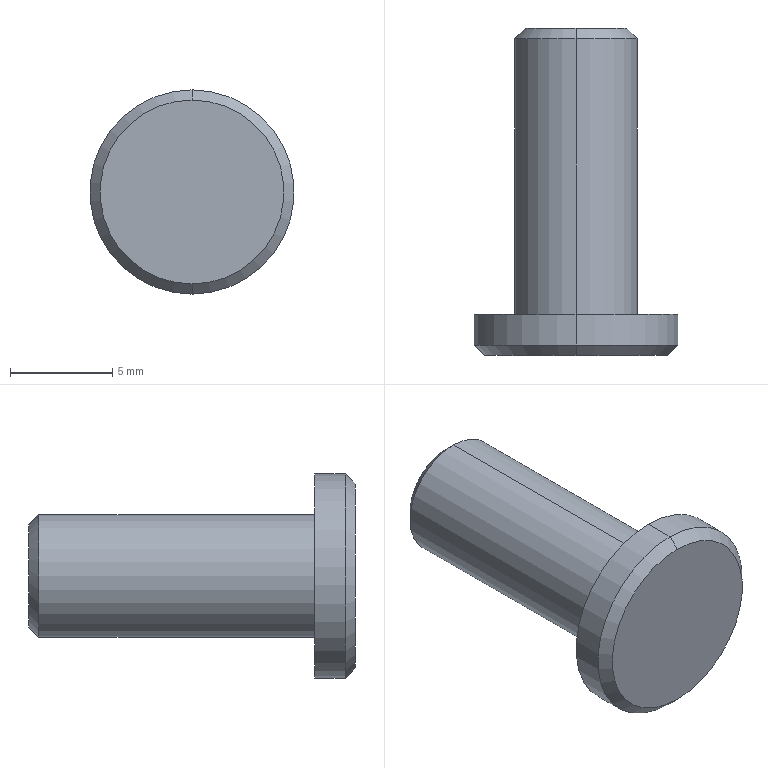Part | SolidWorks | features Chamfer 1, Extrusion 1, ICE 1 | 1 solid | 11 faces | box 10 x 16 x 10 mm | volume 546.899 mm3 | cone 4 | cylinder 4 | plane 3 | commonest cylinder face diameters 6 x2 10 x2
STEP:
#1=CARTESIAN_POINT('',(0.,0.,-4.5));
#2=VERTEX_POINT('',#1);
#3=CARTESIAN_POINT('',(0.,0.,4.5));
#4=VERTEX_POINT('',#3);
#5=CARTESIAN_POINT('',(0.,0.,0.));
#6=DIRECTION('',(0.,-1.,0.));
#7=DIRECTION('',(0.,0.,1.));
#8=AXIS2_PLACEMENT_3D('',#5,#6,#7);
#9=CIRCLE('',#8,4.5);
#10=EDGE_CURVE('',#2,#4,#9,.T.);
#11=ORIENTED_EDGE('',*,*,#10,.F.);
#12=CARTESIAN_POINT('',(0.,0.5,-5.));
#13=VERTEX_POINT('',#12);
#14=CARTESIAN_POINT('',(0.,0.5,-5.));
#15=DIRECTION('',(0.,0.7071,-0.7071));
#16=VECTOR('',#15,1000.);
#17=LINE('',#14,#16);
#18=EDGE_CURVE('',#2,#13,#17,.T.);
#19=ORIENTED_EDGE('',*,*,#18,.T.);
#20=CARTESIAN_POINT('',(0.,0.5,5.));
#21=VERTEX_POINT('',#20);
#22=CARTESIAN_POINT('',(0.,0.5,0.));
#23=DIRECTION('',(0.,1.,0.));
#24=DIRECTION('',(0.,0.,1.));
#25=AXIS2_PLACEMENT_3D('',#22,#23,#24);
#26=CIRCLE('',#25,5.);
#27=EDGE_CURVE('',#21,#13,#26,.T.);
#28=ORIENTED_EDGE('',*,*,#27,.F.);
#29=CARTESIAN_POINT('',(0.,0.5,5.));
#30=DIRECTION('',(0.,0.7071,0.7071));
#31=VECTOR('',#30,1000.);
#32=LINE('',#29,#31);
#33=EDGE_CURVE('',#4,#21,#32,.T.);
#34=ORIENTED_EDGE('',*,*,#33,.F.);
#35=EDGE_LOOP('',(#11,#19,#28,#34));
#36=FACE_OUTER_BOUND('',#35,.T.);
#37=CARTESIAN_POINT('',(0.,0.5,0.));
#38=DIRECTION('',(0.,1.,0.));
#39=DIRECTION('',(0.,0.,1.));
#40=AXIS2_PLACEMENT_3D('',#37,#38,#39);
#41=CONICAL_SURFACE('',#40,5.,0.7854);
#42=ADVANCED_FACE('',(#36),#41,.T.);
#43=CARTESIAN_POINT('',(0.,16.,2.5));
#44=VERTEX_POINT('',#43);
#45=CARTESIAN_POINT('',(0.,16.,-2.5));
#46=VERTEX_POINT('',#45);
#47=CARTESIAN_POINT('',(0.,16.,0.));
#48=DIRECTION('',(0.,1.,0.));
#49=DIRECTION('',(0.,0.,1.));
#50=AXIS2_PLACEMENT_3D('',#47,#48,#49);
#51=CIRCLE('',#50,2.5);
#52=EDGE_CURVE('',#44,#46,#51,.T.);
#53=ORIENTED_EDGE('',*,*,#52,.F.);
#54=CARTESIAN_POINT('',(0.,15.5,3.));
#55=VERTEX_POINT('',#54);
#56=CARTESIAN_POINT('',(0.,16.,2.5));
#57=DIRECTION('',(0.,-0.7071,0.7071));
#58=VECTOR('',#57,1000.);
#59=LINE('',#56,#58);
#60=EDGE_CURVE('',#44,#55,#59,.T.);
#61=ORIENTED_EDGE('',*,*,#60,.T.);
#62=CARTESIAN_POINT('',(0.,15.5,-3.));
#63=VERTEX_POINT('',#62);
#64=CARTESIAN_POINT('',(0.,15.5,0.));
#65=DIRECTION('',(0.,-1.,0.));
#66=DIRECTION('',(0.,0.,1.));
#67=AXIS2_PLACEMENT_3D('',#64,#65,#66);
#68=CIRCLE('',#67,3.);
#69=EDGE_CURVE('',#63,#55,#68,.T.);
#70=ORIENTED_EDGE('',*,*,#69,.F.);
#71=CARTESIAN_POINT('',(0.,16.,-2.5));
#72=DIRECTION('',(0.,-0.7071,-0.7071));
#73=VECTOR('',#72,1000.);
#74=LINE('',#71,#73);
#75=EDGE_CURVE('',#46,#63,#74,.T.);
#76=ORIENTED_EDGE('',*,*,#75,.F.);
#77=EDGE_LOOP('',(#53,#61,#70,#76));
#78=FACE_OUTER_BOUND('',#77,.T.);
#79=CARTESIAN_POINT('',(0.,16.,0.));
#80=DIRECTION('',(0.,-1.,0.));
#81=DIRECTION('',(0.,0.,-1.));
#82=AXIS2_PLACEMENT_3D('',#79,#80,#81);
#83=CONICAL_SURFACE('',#82,2.5,0.7854);
#84=ADVANCED_FACE('',(#78),#83,.T.);
#85=ORIENTED_EDGE('',*,*,#69,.T.);
#86=CARTESIAN_POINT('',(0.,2.,3.));
#87=VERTEX_POINT('',#86);
#88=CARTESIAN_POINT('',(0.,16.,3.));
#89=DIRECTION('',(0.,-1.,0.));
#90=VECTOR('',#89,1000.);
#91=LINE('',#88,#90);
#92=EDGE_CURVE('',#55,#87,#91,.T.);
#93=ORIENTED_EDGE('',*,*,#92,.T.);
#94=CARTESIAN_POINT('',(0.,2.,-3.));
#95=VERTEX_POINT('',#94);
#96=CARTESIAN_POINT('',(0.,2.,0.));
#97=DIRECTION('',(0.,1.,0.));
#98=DIRECTION('',(0.,0.,1.));
#99=AXIS2_PLACEMENT_3D('',#96,#97,#98);
#100=CIRCLE('',#99,3.);
#101=EDGE_CURVE('',#87,#95,#100,.T.);
#102=ORIENTED_EDGE('',*,*,#101,.T.);
#103=CARTESIAN_POINT('',(0.,16.,-3.));
#104=DIRECTION('',(0.,-1.,0.));
#105=VECTOR('',#104,1000.);
#106=LINE('',#103,#105);
#107=EDGE_CURVE('',#63,#95,#106,.T.);
#108=ORIENTED_EDGE('',*,*,#107,.F.);
#109=EDGE_LOOP('',(#85,#93,#102,#108));
#110=FACE_OUTER_BOUND('',#109,.T.);
#111=CARTESIAN_POINT('',(0.,16.,0.));
#112=DIRECTION('',(0.,-1.,0.));
#113=DIRECTION('',(0.,0.,-1.));
#114=AXIS2_PLACEMENT_3D('',#111,#112,#113);
#115=CYLINDRICAL_SURFACE('',#114,3.);
#116=ADVANCED_FACE('',(#110),#115,.T.);
#117=CARTESIAN_POINT('',(0.,2.,5.));
#118=VERTEX_POINT('',#117);
#119=CARTESIAN_POINT('',(0.,2.,-5.));
#120=VERTEX_POINT('',#119);
#121=CARTESIAN_POINT('',(0.,2.,0.));
#122=DIRECTION('',(0.,1.,0.));
#123=DIRECTION('',(0.,0.,1.));
#124=AXIS2_PLACEMENT_3D('',#121,#122,#123);
#125=CIRCLE('',#124,5.);
#126=EDGE_CURVE('',#118,#120,#125,.T.);
#127=ORIENTED_EDGE('',*,*,#126,.F.);
#128=CARTESIAN_POINT('',(0.,2.,5.));
#129=DIRECTION('',(0.,-1.,0.));
#130=VECTOR('',#129,1000.);
#131=LINE('',#128,#130);
#132=EDGE_CURVE('',#118,#21,#131,.T.);
#133=ORIENTED_EDGE('',*,*,#132,.T.);
#134=ORIENTED_EDGE('',*,*,#27,.T.);
#135=CARTESIAN_POINT('',(0.,2.,-5.));
#136=DIRECTION('',(0.,-1.,0.));
#137=VECTOR('',#136,1000.);
#138=LINE('',#135,#137);
#139=EDGE_CURVE('',#120,#13,#138,.T.);
#140=ORIENTED_EDGE('',*,*,#139,.F.);
#141=EDGE_LOOP('',(#127,#133,#134,#140));
#142=FACE_OUTER_BOUND('',#141,.T.);
#143=CARTESIAN_POINT('',(0.,2.,0.));
#144=DIRECTION('',(0.,-1.,0.));
#145=DIRECTION('',(0.,0.,-1.));
#146=AXIS2_PLACEMENT_3D('',#143,#144,#145);
#147=CYLINDRICAL_SURFACE('',#146,5.);
#148=ADVANCED_FACE('',(#142),#147,.T.);
#149=ORIENTED_EDGE('',*,*,#132,.F.);
#150=CARTESIAN_POINT('',(0.,2.,0.));
#151=DIRECTION('',(0.,1.,0.));
#152=DIRECTION('',(0.,0.,1.));
#153=AXIS2_PLACEMENT_3D('',#150,#151,#152);
#154=CIRCLE('',#153,5.);
#155=EDGE_CURVE('',#120,#118,#154,.T.);
#156=ORIENTED_EDGE('',*,*,#155,.F.);
#157=ORIENTED_EDGE('',*,*,#139,.T.);
#158=CARTESIAN_POINT('',(0.,0.5,0.));
#159=DIRECTION('',(0.,1.,0.));
#160=DIRECTION('',(0.,0.,1.));
#161=AXIS2_PLACEMENT_3D('',#158,#159,#160);
#162=CIRCLE('',#161,5.);
#163=EDGE_CURVE('',#13,#21,#162,.T.);
#164=ORIENTED_EDGE('',*,*,#163,.T.);
#165=EDGE_LOOP('',(#149,#156,#157,#164));
#166=FACE_OUTER_BOUND('',#165,.T.);
#167=CARTESIAN_POINT('',(0.,2.,0.));
#168=DIRECTION('',(0.,-1.,0.));
#169=DIRECTION('',(0.,0.,-1.));
#170=AXIS2_PLACEMENT_3D('',#167,#168,#169);
#171=CYLINDRICAL_SURFACE('',#170,5.);
#172=ADVANCED_FACE('',(#166),#171,.T.);
#173=CARTESIAN_POINT('',(0.,2.,0.));
#174=DIRECTION('',(0.,1.,0.));
#175=DIRECTION('',(0.,0.,1.));
#176=AXIS2_PLACEMENT_3D('',#173,#174,#175);
#177=CIRCLE('',#176,3.);
#178=EDGE_CURVE('',#95,#87,#177,.T.);
#179=ORIENTED_EDGE('',*,*,#178,.F.);
#180=ORIENTED_EDGE('',*,*,#101,.F.);
#181=EDGE_LOOP('',(#179,#180));
#182=FACE_BOUND('',#181,.T.);
#183=ORIENTED_EDGE('',*,*,#155,.T.);
#184=ORIENTED_EDGE('',*,*,#126,.T.);
#185=EDGE_LOOP('',(#183,#184));
#186=FACE_OUTER_BOUND('',#185,.T.);
#187=CARTESIAN_POINT('',(0.,2.,0.));
#188=DIRECTION('',(0.,1.,0.));
#189=DIRECTION('',(0.,0.,1.));
#190=AXIS2_PLACEMENT_3D('',#187,#188,#189);
#191=PLANE('',#190);
#192=ADVANCED_FACE('',(#182,#186),#191,.T.);
#193=CARTESIAN_POINT('',(0.,0.,0.));
#194=DIRECTION('',(0.,-1.,0.));
#195=DIRECTION('',(0.,0.,1.));
#196=AXIS2_PLACEMENT_3D('',#193,#194,#195);
#197=CIRCLE('',#196,4.5);
#198=EDGE_CURVE('',#4,#2,#197,.T.);
#199=ORIENTED_EDGE('',*,*,#198,.T.);
#200=ORIENTED_EDGE('',*,*,#10,.T.);
#201=EDGE_LOOP('',(#199,#200));
#202=FACE_OUTER_BOUND('',#201,.T.);
#203=CARTESIAN_POINT('',(0.,0.,0.));
#204=DIRECTION('',(0.,1.,0.));
#205=DIRECTION('',(0.,0.,1.));
#206=AXIS2_PLACEMENT_3D('',#203,#204,#205);
#207=PLANE('',#206);
#208=ADVANCED_FACE('',(#202),#207,.F.);
#209=ORIENTED_EDGE('',*,*,#92,.F.);
#210=CARTESIAN_POINT('',(0.,15.5,0.));
#211=DIRECTION('',(0.,-1.,0.));
#212=DIRECTION('',(0.,0.,1.));
#213=AXIS2_PLACEMENT_3D('',#210,#211,#212);
#214=CIRCLE('',#213,3.);
#215=EDGE_CURVE('',#55,#63,#214,.T.);
#216=ORIENTED_EDGE('',*,*,#215,.T.);
#217=ORIENTED_EDGE('',*,*,#107,.T.);
#218=ORIENTED_EDGE('',*,*,#178,.T.);
#219=EDGE_LOOP('',(#209,#216,#217,#218));
#220=FACE_OUTER_BOUND('',#219,.T.);
#221=CARTESIAN_POINT('',(0.,16.,0.));
#222=DIRECTION('',(0.,-1.,0.));
#223=DIRECTION('',(0.,0.,-1.));
#224=AXIS2_PLACEMENT_3D('',#221,#222,#223);
#225=CYLINDRICAL_SURFACE('',#224,3.);
#226=ADVANCED_FACE('',(#220),#225,.T.);
#227=CARTESIAN_POINT('',(0.,16.,0.));
#228=DIRECTION('',(0.,1.,0.));
#229=DIRECTION('',(0.,0.,1.));
#230=AXIS2_PLACEMENT_3D('',#227,#228,#229);
#231=CIRCLE('',#230,2.5);
#232=EDGE_CURVE('',#46,#44,#231,.T.);
#233=ORIENTED_EDGE('',*,*,#232,.T.);
#234=ORIENTED_EDGE('',*,*,#52,.T.);
#235=EDGE_LOOP('',(#233,#234));
#236=FACE_OUTER_BOUND('',#235,.T.);
#237=CARTESIAN_POINT('',(0.,16.,0.));
#238=DIRECTION('',(0.,1.,0.));
#239=DIRECTION('',(0.,0.,1.));
#240=AXIS2_PLACEMENT_3D('',#237,#238,#239);
#241=PLANE('',#240);
#242=ADVANCED_FACE('',(#236),#241,.T.);
#243=ORIENTED_EDGE('',*,*,#60,.F.);
#244=ORIENTED_EDGE('',*,*,#232,.F.);
#245=ORIENTED_EDGE('',*,*,#75,.T.);
#246=ORIENTED_EDGE('',*,*,#215,.F.);
#247=EDGE_LOOP('',(#243,#244,#245,#246));
#248=FACE_OUTER_BOUND('',#247,.T.);
#249=CARTESIAN_POINT('',(0.,16.,0.));
#250=DIRECTION('',(0.,-1.,0.));
#251=DIRECTION('',(0.,0.,-1.));
#252=AXIS2_PLACEMENT_3D('',#249,#250,#251);
#253=CONICAL_SURFACE('',#252,2.5,0.7854);
#254=ADVANCED_FACE('',(#248),#253,.T.);
#255=ORIENTED_EDGE('',*,*,#18,.F.);
#256=ORIENTED_EDGE('',*,*,#198,.F.);
#257=ORIENTED_EDGE('',*,*,#33,.T.);
#258=ORIENTED_EDGE('',*,*,#163,.F.);
#259=EDGE_LOOP('',(#255,#256,#257,#258));
#260=FACE_OUTER_BOUND('',#259,.T.);
#261=CARTESIAN_POINT('',(0.,0.5,0.));
#262=DIRECTION('',(0.,1.,0.));
#263=DIRECTION('',(0.,0.,1.));
#264=AXIS2_PLACEMENT_3D('',#261,#262,#263);
#265=CONICAL_SURFACE('',#264,5.,0.7854);
#266=ADVANCED_FACE('',(#260),#265,.T.);
#267=CLOSED_SHELL('',(#42,#84,#116,#148,#172,#192,#208,#226,#242,#254,#266));
#268=MANIFOLD_SOLID_BREP('',#267);
#269=CARTESIAN_POINT('',(0.,0.,0.));
#270=DIRECTION('',(0.,0.,1.));
#271=DIRECTION('',(1.,0.,0.));
#272=AXIS2_PLACEMENT_3D('',#269,#270,#271);
#273=(LENGTH_UNIT()NAMED_UNIT(*)SI_UNIT(.MILLI.,.METRE.));
#274=UNCERTAINTY_MEASURE_WITH_UNIT(LENGTH_MEASURE(0.00001),#273,'','');
#275=(NAMED_UNIT(*)PLANE_ANGLE_UNIT()SI_UNIT($,.RADIAN.));
#276=(NAMED_UNIT(*)SI_UNIT($,.STERADIAN.)SOLID_ANGLE_UNIT());
#277=(GEOMETRIC_REPRESENTATION_CONTEXT(3)GLOBAL_UNCERTAINTY_ASSIGNED_CONTEXT((#274))GLOBAL_UNIT_ASSIGNED_CONTEXT((#273,#275,#276))REPRESENTATION_CONTEXT('',''));
#278=ADVANCED_BREP_SHAPE_REPRESENTATION('',(#268,#272),#277);